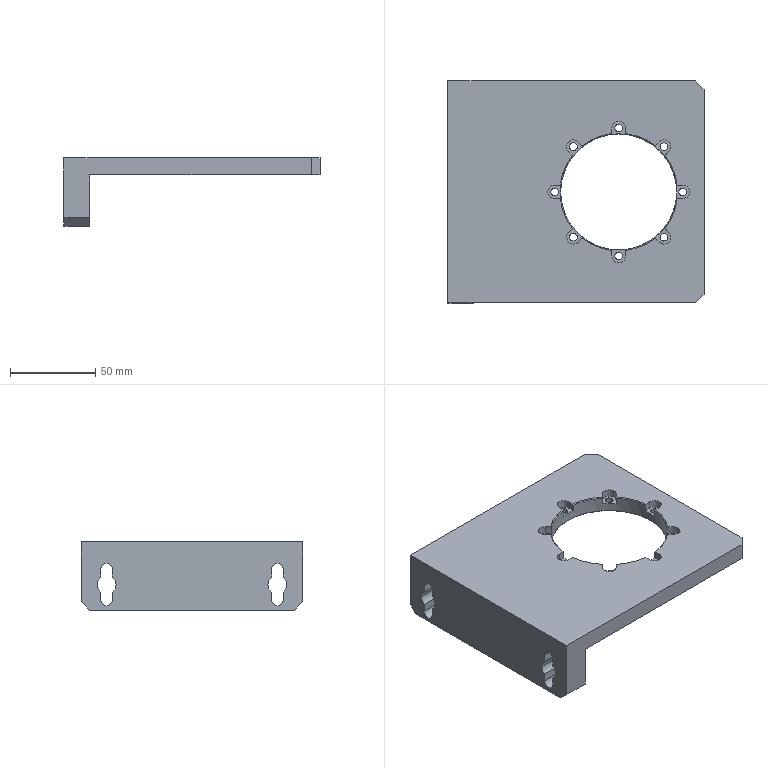NC program | NX | posted with a generic post | part box 150 x 130 x 40 mm
Lines 1321 to 2441 of 2441:
(ZLEVEL_PROFILE , TOOL : D6)
N2610 T12 M6
N2612 G54
N2614 G17 G0 G90 X55.46 Y0. B0. C0. S9500 M3
N2616 G43 Z30. H12
N2618 Z-0.46
N2620 G94 G1 X56.598 Y-0.705 F2000.
N2622 G3 X57.119 Y-1.004 R0.6
N2624 G1 X58.842 Y-1.
N2626 X62.5
N2628 G3 X63.5 Y0. R1.
N2630 X62.5 Y1. R1.
N2632 G1 X58.764 Y1.003
N2634 X57.118 Y1.004
N2636 G3 X56.598 Y0.704 R0.6
N2638 G1 X55.46 Y0.
N2640 G0 X55.455 Z-0.92
N2642 G1 X56.571 Y-0.704
N2644 G3 X57.091 Y-1.003 R0.6
N2646 G1 X58.842 Y-1.
N2648 X62.5
N2650 G3 X63.5 Y0. R1.
N2652 X62.5 Y1. R1.
N2654 G1 X58.764
N2656 X57.09 Y1.003
N2658 G3 X56.57 Y0.704 R0.6
N2660 G1 X55.455 Y0.
N2662 G0 X55.459 Z-1.38
N2664 G1 X56.543 Y-0.704
N2666 G3 X57.063 Y-1.003 R0.6
N2668 G1 X58.842 Y-1.
N2670 X62.5
N2672 G3 X63.5 Y0. R1.
N2674 X62.5 Y1. R1.
N2676 G1 X58.764
N2678 X57.062 Y1.003
N2680 G3 X56.542 Y0.704 R0.6
N2682 G1 X55.459 Y0.
N2684 G0 X55.462 Z-1.84
N2686 G1 X56.516 Y-0.703
N2688 G3 X57.036 Y-1.003 R0.6
N2690 G1 X58.842 Y-1.
N2692 X62.5
N2694 G3 X63.5 Y0. R1.
N2696 X62.5 Y1. R1.
N2698 G1 X58.764
N2700 X57.034 Y1.003
N2702 G3 X56.514 Y0.703 R0.6
N2704 G1 X55.462 Y0.
N2706 G0 X55.465 Z-2.3
N2708 G1 X56.488 Y-0.703
N2710 G3 X57.008 Y-1.002 R0.6
N2712 G1 X58.842 Y-1.
N2714 X62.5
N2716 G3 X63.5 Y0. R1.
N2718 X62.5 Y1. R1.
N2720 G1 X58.764
N2722 X57.007 Y1.002
N2724 G3 X56.487 Y0.703 R0.6
N2726 G1 X55.465 Y0.
N2728 G0 X55.467 Z-2.76
N2730 G1 X56.46 Y-0.703
N2732 G3 X56.98 Y-1.002 R0.6
N2734 G1 X58.842 Y-1.
N2736 X62.5
N2738 G3 X63.5 Y0. R1.
N2740 X62.5 Y1. R1.
N2742 G1 X58.764
N2744 X56.979 Y1.002
N2746 G3 X56.459 Y0.703 R0.6
N2748 G1 X55.467 Y0.
N2750 G0 X55.47 Z-3.22
N2752 G1 X56.433 Y-0.702
N2754 G3 X56.953 Y-1.002 R0.6
N2756 G1 X58.842 Y-1.
N2758 X62.5
N2760 G3 X63.5 Y0. R1.
N2762 X62.5 Y1. R1.
N2764 G1 X58.764
N2766 X56.951 Y1.002
N2768 G3 X56.431 Y0.702 R0.6
N2770 G1 X55.47 Y0.
N2772 G0 X55.471 Z-3.68
N2774 G1 X56.405 Y-0.702
N2776 G3 X56.925 Y-1.001 R0.6
N2778 G1 X58.842 Y-1.
N2780 X62.5
N2782 G3 X63.5 Y0. R1.
N2784 X62.5 Y1. R1.
N2786 G1 X58.764
N2788 X56.923 Y1.001
N2790 G3 X56.403 Y0.702 R0.6
N2792 G1 X55.471 Y0.
N2794 G0 X55.472 Z-4.14
N2796 G1 X56.377 Y-0.701
N2798 G3 X56.897 Y-1.001 R0.6
N2800 G1 X58.88 Y-1.
N2802 X62.5
N2804 G3 X63.5 Y0. R1.
N2806 X62.5 Y1. R1.
N2808 G1 X58.764
N2810 X56.895 Y1.001
N2812 G3 X56.375 Y0.701 R0.6
N2814 G1 X55.472 Y0.
N2816 G0 X55.471 Z-4.6
N2818 G1 X56.35 Y-0.701
N2820 G3 X56.87 Y-1.001 R0.6
N2822 G1 X58.88 Y-1.
N2824 X62.5
N2826 G3 X63.5 Y0. R1.
N2828 X62.5 Y1. R1.
N2830 G1 X58.764
N2832 X56.867 Y1.001
N2834 G3 X56.348 Y0.701 R0.6
N2836 G1 X55.471 Y0.
N2838 G0 Z30.
N2840 X46.559 Y21.559
N2842 Z-0.46
N2844 G1 X47.579 Y21.583
N2846 G3 X48.158 Y21.74 R0.6
N2848 G1 X49.644 Y23.229
N2850 X52.224 Y25.809
N2852 G3 X52.224 Y27.224 R1.
N2854 X50.809 Y27.224 R1.
N2856 G1 X48.19 Y24.604
N2858 X48.165 Y24.584
N2860 X46.741 Y23.16
N2862 G3 X46.586 Y22.58 R0.6
N2864 G1 X46.559 Y21.559
N2866 G0 X46.558 Y21.558 Z-0.92
N2868 G1 X47.579 Y21.584
N2870 G3 X48.158 Y21.74 R0.6
N2872 G1 X49.644 Y23.229
N2874 X52.224 Y25.809
N2876 G3 X52.224 Y27.224 R1.
N2878 X50.809 Y27.224 R1.
N2880 G1 X48.168 Y24.582
N2882 X46.742 Y23.159
N2884 G3 X46.586 Y22.58 R0.6
N2886 G1 X46.558 Y21.558
N2888 G0 X46.557 Y21.557 Z-1.38
N2890 G1 X47.578 Y21.584
N2892 G3 X48.158 Y21.74 R0.6
N2894 G1 X49.644 Y23.229
N2896 X52.224 Y25.809
N2898 G3 X52.224 Y27.224 R1.
N2900 X50.809 Y27.224 R1.
N2902 G1 X48.168 Y24.582
N2904 X46.742 Y23.159
N2906 G3 X46.586 Y22.58 R0.6
N2908 G1 X46.557 Y21.557
N2910 G0 X46.556 Y21.556 Z-1.84
N2912 G1 X47.578 Y21.585
N2914 G3 X48.157 Y21.74 R0.6
N2916 G1 X49.644 Y23.229
N2918 X52.224 Y25.809
N2920 G3 X52.224 Y27.224 R1.
N2922 X50.809 Y27.224 R1.
N2924 G1 X48.168 Y24.582
N2926 X46.753 Y23.169
N2928 G3 X46.597 Y22.59 R0.6
N2930 G1 X46.556 Y21.556
N2932 G0 X46.555 Y21.555 Z-2.3
N2934 G1 X47.578 Y21.585
N2936 G3 X48.157 Y21.741 R0.6
N2938 G1 X49.665 Y23.251
N2940 X52.224 Y25.809
N2942 G3 X52.224 Y27.224 R1.
N2944 X50.809 Y27.224 R1.
N2946 G1 X48.168 Y24.582
N2948 X46.753 Y23.169
N2950 G3 X46.598 Y22.589 R0.6
N2952 G1 X46.555 Y21.555
N2954 G0 X46.554 Y21.553 Z-2.76
N2956 G1 X47.577 Y21.586
N2958 G3 X48.157 Y21.741 R0.6
N2960 G1 X49.665 Y23.251
N2962 X52.224 Y25.809
N2964 G3 X52.224 Y27.224 R1.
N2966 X50.809 Y27.224 R1.
N2968 G1 X48.168 Y24.582
N2970 X46.754 Y23.168
N2972 G3 X46.598 Y22.589 R0.6
N2974 G1 X46.554 Y21.553
N2976 G0 X46.55 Y21.551 Z-3.22
N2978 G1 X47.577 Y21.586
N2980 G3 X48.156 Y21.741 R0.6
N2982 G1 X49.665 Y23.251
N2984 X52.224 Y25.809
N2986 G3 X52.224 Y27.224 R1.
N2988 X50.809 Y27.224 R1.
N2990 G1 X48.168 Y24.582
N2992 X46.754 Y23.168
N2994 G3 X46.599 Y22.588 R0.6
N2996 G1 X46.55 Y21.551
N2998 G0 X46.549 Y21.55 Z-3.68
N3000 G1 X47.576 Y21.586
N3002 G3 X48.156 Y21.742 R0.6
N3004 G1 X49.665 Y23.251
N3006 X52.224 Y25.809
N3008 G3 X52.224 Y27.224 R1.
N3010 X50.809 Y27.224 R1.
N3012 G1 X48.168 Y24.582
N3014 X46.754 Y23.168
N3016 G3 X46.599 Y22.588 R0.6
N3018 G1 X46.549 Y21.55
N3020 G0 X46.55 Z-4.14
N3022 G1 X47.576 Y21.587
N3024 G3 X48.156 Y21.742 R0.6
N3026 G1 X49.665 Y23.251
N3028 X52.224 Y25.809
N3030 G3 X52.224 Y27.224 R1.
N3032 X50.809 Y27.224 R1.
N3034 G1 X48.168 Y24.582
N3036 X46.755 Y23.167
N3038 G3 X46.6 Y22.588 R0.6
N3040 G1 X46.55 Y21.55
N3042 G0 X46.548 Y21.548 Z-4.6
N3044 G1 X47.586 Y21.598
N3046 G3 X48.166 Y21.753 R0.6
N3048 G1 X49.665 Y23.251
N3050 X52.224 Y25.809
N3052 G3 X52.224 Y27.224 R1.
N3054 X50.809 Y27.224 R1.
N3056 G1 X48.168 Y24.582
N3058 X46.755 Y23.167
N3060 G3 X46.6 Y22.587 R0.6
N3062 G1 X46.548 Y21.548
N3064 G0 Z30.
N3066 X25. Y30.46
N3068 Z-0.46
N3070 G1 X25.705 Y31.598
N3072 G3 X26.004 Y32.118 R0.6
N3074 G1 X26. Y33.991
N3076 Y37.5
N3078 G3 X25. Y38.5 R1.
N3080 X24. Y37.5 R1.
N3082 G1 Y33.991
N3084 X23.996 Y32.118
N3086 G3 X24.295 Y31.598 R0.6
N3088 G1 X25. Y30.46
N3090 G0 Y30.454 Z-0.92
N3092 G1 X25.704 Y31.57
N3094 G3 X26.003 Y32.09 R0.6
N3096 G1 X26. Y33.991
N3098 Y37.5
N3100 G3 X25. Y38.5 R1.
N3102 X24. Y37.5 R1.
N3104 G1 Y33.991
N3106 X23.997 Y32.09
N3108 G3 X24.296 Y31.57 R0.6
N3110 G1 X25. Y30.454
N3112 G0 Y30.459 Z-1.38
N3114 G1 X25.704 Y31.542
N3116 G3 X26.003 Y32.062 R0.6
N3118 G1 X26. Y33.991
N3120 Y37.5
N3122 G3 X25. Y38.5 R1.
N3124 X24. Y37.5 R1.
N3126 G1 Y33.991
N3128 X23.997 Y32.062
N3130 G3 X24.296 Y31.542 R0.6
N3132 G1 X25. Y30.459
N3134 G0 Y30.462 Z-1.84
N3136 G1 X25.703 Y31.514
N3138 G3 X26.003 Y32.034 R0.6
N3140 G1 X26. Y33.991
N3142 Y37.5
N3144 G3 X25. Y38.5 R1.
N3146 X24. Y37.5 R1.
N3148 G1 Y33.991
N3150 X23.997 Y32.034
N3152 G3 X24.297 Y31.514 R0.6
N3154 G1 X25. Y30.462
N3156 G0 Y30.466 Z-2.3
N3158 G1 X25.703 Y31.487
N3160 G3 X26.002 Y32.007 R0.6
N3162 G1 X26. Y33.991
N3164 Y37.5
N3166 G3 X25. Y38.5 R1.
N3168 X24. Y37.5 R1.
N3170 G1 Y33.991
N3172 X23.998 Y32.007
N3174 G3 X24.297 Y31.487 R0.6
N3176 G1 X25. Y30.466
N3178 G0 Y30.467 Z-2.76
N3180 G1 X25.702 Y31.459
N3182 G3 X26.002 Y31.979 R0.6
N3184 G1 X26. Y33.991
N3186 Y37.5
N3188 G3 X25. Y38.5 R1.
N3190 X24. Y37.5 R1.
N3192 G1 Y33.991
N3194 X23.998 Y31.979
N3196 G3 X24.298 Y31.459 R0.6
N3198 G1 X25. Y30.467
N3200 G0 Y30.47 Z-3.22
N3202 G1 X25.702 Y31.431
N3204 G3 X26.002 Y31.951 R0.6
N3206 G1 X26. Y33.991
N3208 Y37.5
N3210 G3 X25. Y38.5 R1.
N3212 X24. Y37.5 R1.
N3214 G1 Y33.991
N3216 X23.998 Y31.951
N3218 G3 X24.298 Y31.431 R0.6
N3220 G1 X25. Y30.47
N3222 G0 Y30.471 Z-3.68
N3224 G1 X25.702 Y31.403
N3226 G3 X26.001 Y31.923 R0.6
N3228 G1 X26. Y33.991
N3230 Y37.5
N3232 G3 X25. Y38.5 R1.
N3234 X24. Y37.5 R1.
N3236 G1 Y33.991
N3238 X23.999 Y31.923
N3240 G3 X24.298 Y31.403 R0.6
N3242 G1 X25. Y30.471
N3244 G0 Y30.472 Z-4.14
N3246 G1 X25.701 Y31.375
N3248 G3 X26.001 Y31.895 R0.6
N3250 G1 X26. Y33.991
N3252 Y37.5
N3254 G3 X25. Y38.5 R1.
N3256 X24. Y37.5 R1.
N3258 G1 Y33.991
N3260 X23.999 Y31.895
N3262 G3 X24.299 Y31.375 R0.6
N3264 G1 X25. Y30.472
N3266 G0 Y30.471 Z-4.6
N3268 G1 X25.701 Y31.348
N3270 G3 X26.001 Y31.867 R0.6
N3272 G1 X26. Y33.991
N3274 Y37.5
N3276 G3 X25. Y38.5 R1.
N3278 X24. Y37.5 R1.
N3280 G1 Y33.991
N3282 X23.999 Y31.867
N3284 G3 X24.299 Y31.348 R0.6
N3286 G1 X25. Y30.471
N3288 G0 Z30.
N3290 X3.439 Y21.56
N3292 Z-0.46
N3294 G1 X3.416 Y22.579
N3296 G3 X3.26 Y23.159 R0.6
N3298 G1 X1.939 Y24.48
N3300 X1.821 Y24.593
N3302 X-0.809 Y27.224
N3304 G3 X-2.224 Y27.224 R1.
N3306 X-2.224 Y25.809 R1.
N3308 G1 X0.396 Y23.19
N3310 X0.416 Y23.165
N3312 X1.84 Y21.74
N3314 G3 X2.42 Y21.584 R0.6
N3316 G1 X3.439 Y21.56
N3318 G0 X3.44 Y21.559 Z-0.92
N3320 G1 X3.415 Y22.579
N3322 G3 X3.26 Y23.158 R0.6
N3324 G1 X1.96 Y24.458
N3326 X1.832 Y24.582
N3328 X-0.809 Y27.224
N3330 G3 X-2.224 Y27.224 R1.
N3332 X-2.224 Y25.809 R1.
N3334 G1 X0.418 Y23.168
N3336 X1.84 Y21.74
N3338 G3 X2.42 Y21.584 R0.6
N3340 G1 X3.44 Y21.559
N3342 G0 X3.442 Y21.558 Z-1.38
N3344 G1 X3.415 Y22.579
N3346 G3 X3.26 Y23.158 R0.6
N3348 G1 X1.959 Y24.458
N3350 X1.832 Y24.582
N3352 X-0.809 Y27.224
N3354 G3 X-2.224 Y27.224 R1.
N3356 X-2.224 Y25.809 R1.
N3358 G1 X0.418 Y23.168
N3360 X1.841 Y21.741
N3362 G3 X2.42 Y21.584 R0.6
N3364 G1 X3.442 Y21.558
N3366 G0 X3.443 Y21.557 Z-1.84
N3368 G1 X3.415 Y22.578
N3370 G3 X3.259 Y23.158 R0.6
N3372 G1 X1.832 Y24.582
N3374 X-0.809 Y27.224
N3376 G3 X-2.224 Y27.224 R1.
N3378 X-2.224 Y25.809 R1.
N3380 G1 X0.418 Y23.168
N3382 X1.841 Y21.741
N3384 G3 X2.42 Y21.585 R0.6
N3386 G1 X3.443 Y21.557
N3388 G0 X3.444 Y21.556 Z-2.3
N3390 G1 X3.415 Y22.578
N3392 G3 X3.259 Y23.157 R0.6
N3394 G1 X1.832 Y24.582
N3396 X-0.809 Y27.224
N3398 G3 X-2.224 Y27.224 R1.
N3400 X-2.224 Y25.809 R1.
N3402 G1 X0.418 Y23.168
N3404 X1.841 Y21.741
N3406 G3 X2.421 Y21.585 R0.6
N3408 G1 X3.444 Y21.556
N3410 G0 X3.445 Y21.555 Z-2.76
N3412 G1 X3.414 Y22.578
N3414 G3 X3.259 Y23.157 R0.6
N3416 G1 X1.832 Y24.582
N3418 X-0.809 Y27.224
N3420 G3 X-2.224 Y27.224 R1.
N3422 X-2.224 Y25.809 R1.
N3424 G1 X0.418 Y23.168
N3426 X1.842 Y21.741
N3428 G3 X2.421 Y21.586 R0.6
N3430 G1 X3.445 Y21.555
N3432 G0 X3.447 Y21.551 Z-3.22
N3434 G1 X3.414 Y22.577
N3436 G3 X3.259 Y23.157 R0.6
N3438 G1 X1.832 Y24.582
N3440 X-0.809 Y27.224
N3442 G3 X-2.224 Y27.224 R1.
N3444 X-2.224 Y25.809 R1.
N3446 G1 X0.418 Y23.168
N3448 X1.842 Y21.742
N3450 G3 X2.422 Y21.586 R0.6
N3452 G1 X3.447 Y21.551
N3454 G0 X3.448 Y21.55 Z-3.68
N3456 G1 X3.403 Y22.587
N3458 G3 X3.247 Y23.167 R0.6
N3460 G1 X1.832 Y24.582
N3462 X-0.809 Y27.224
N3464 G3 X-2.224 Y27.224 R1.
N3466 X-2.224 Y25.809 R1.
N3468 G1 X0.418 Y23.168
N3470 X1.843 Y21.742
N3472 G3 X2.422 Y21.587 R0.6
N3474 G1 X3.448 Y21.55
N3476 G0 X3.449 Y21.551 Z-4.14
N3478 G1 X3.402 Y22.587
N3480 G3 X3.247 Y23.167 R0.6
N3482 G1 X1.832 Y24.582
N3484 X-0.809 Y27.224
N3486 G3 X-2.224 Y27.224 R1.
N3488 X-2.224 Y25.809 R1.
N3490 G1 X0.418 Y23.168
N3492 X1.832 Y21.753
N3494 G3 X2.412 Y21.598 R0.6
N3496 G1 X3.449 Y21.551
N3498 G0 X3.45 Y21.55 Z-4.6
N3500 G1 X3.402 Y22.587
N3502 G3 X3.247 Y23.166 R0.6
N3504 G1 X1.832 Y24.582
N3506 X-0.809 Y27.224
N3508 G3 X-2.224 Y27.224 R1.
N3510 X-2.224 Y25.809 R1.
N3512 G1 X0.418 Y23.168
N3514 X1.833 Y21.753
N3516 G3 X2.412 Y21.598 R0.6
N3518 G1 X3.45 Y21.55
N3520 G0 Z30.
N3522 X-5.46 Y0.
N3524 Z-0.46
N3526 G1 X-6.599 Y0.705
N3528 G3 X-7.119 Y1.004 R0.6
N3530 G1 X-8.742 Y1.
N3532 X-12.5
N3534 G3 X-13.5 Y0. R1.
N3536 X-12.5 Y-1. R1.
N3538 G1 X-8.764 Y-1.003
N3540 X-7.118 Y-1.004
N3542 G3 X-6.598 Y-0.704 R0.6
N3544 G1 X-5.46 Y0.
N3546 G0 X-5.462 Y0.002 Z-0.92
N3548 G1 X-6.571 Y0.704
N3550 G3 X-7.091 Y1.003 R0.6
N3552 G1 X-8.718 Y1.
N3554 X-12.5
N3556 G3 X-13.5 Y0. R1.
N3558 X-12.5 Y-1. R1.
N3560 G1 X-8.764
N3562 X-8.182 Y-1.057
N3564 X-8.134 Y-1.002
N3566 X-7.09 Y-1.003
N3568 G3 X-6.57 Y-0.704 R0.6
N3570 G1 X-5.462 Y0.002
N3572 G0 X-5.465 Y0.001 Z-1.38
N3574 G1 X-6.543 Y0.704
N3576 G3 X-7.063 Y1.003 R0.6
N3578 G1 X-8.718 Y1.
N3580 X-12.5
N3582 G3 X-13.5 Y0. R1.
N3584 X-12.5 Y-1. R1.
N3586 G1 X-8.764
N3588 X-8.182 Y-1.057
N3590 X-8.134 Y-1.002
N3592 X-7.062 Y-1.003
N3594 G3 X-6.543 Y-0.703 R0.6
N3596 G1 X-5.465 Y0.001
N3598 G0 X-5.468 Z-1.84
N3600 G1 X-6.516 Y0.703
N3602 G3 X-7.036 Y1.003 R0.6
N3604 G1 X-8.718 Y1.
N3606 X-12.5
N3608 G3 X-13.5 Y0. R1.
N3610 X-12.5 Y-1. R1.
N3612 G1 X-8.764
N3614 X-8.182 Y-1.057
N3616 X-8.134 Y-1.002
N3618 X-7.035 Y-1.003
N3620 G3 X-6.515 Y-0.703 R0.6
N3622 G1 X-5.468 Y0.001
N3624 G0 X-5.469 Z-2.3
N3626 G1 X-6.488 Y0.703
N3628 G3 X-7.008 Y1.002 R0.6
N3630 G1 X-8.718 Y1.
N3632 X-12.5
N3634 G3 X-13.5 Y0. R1.
N3636 X-12.5 Y-1. R1.
N3638 G1 X-8.764
N3640 X-8.182 Y-1.057
N3642 X-8.134 Y-1.001
N3644 X-7.007 Y-1.002
N3646 G3 X-6.487 Y-0.703 R0.6
N3648 G1 X-5.469 Y0.001
N3650 G0 X-5.471 Y0. Z-2.76
N3652 G1 X-6.46 Y0.703
N3654 G3 X-6.98 Y1.002 R0.6
N3656 G1 X-8.718 Y1.
N3658 X-12.5
N3660 G3 X-13.5 Y0. R1.
N3662 X-12.5 Y-1. R1.
N3664 G1 X-8.764
N3666 X-8.182 Y-1.057
N3668 X-8.134 Y-1.001
N3670 X-6.979 Y-1.002
N3672 G3 X-6.459 Y-0.703 R0.6
N3674 G1 X-5.471 Y0.
N3676 G0 X-5.473 Z-3.22
N3678 G1 X-6.433 Y0.702
N3680 G3 X-6.953 Y1.002 R0.6
N3682 G1 X-8.718 Y1.
N3684 X-12.5
N3686 G3 X-13.5 Y0. R1.
N3688 X-12.5 Y-1. R1.
N3690 G1 X-8.764
N3692 X-8.182 Y-1.057
N3694 X-8.134 Y-1.
N3696 X-6.951 Y-1.002
N3698 G3 X-6.431 Y-0.702 R0.6
N3700 G1 X-5.473 Y0.
N3702 G0 X-5.476 Y-0.001 Z-3.68
N3704 G1 X-6.405 Y0.702
N3706 G3 X-6.925 Y1.001 R0.6
N3708 G1 X-8.718 Y1.
N3710 X-12.5
N3712 G3 X-13.5 Y0. R1.
N3714 X-12.5 Y-1. R1.
N3716 G1 X-8.764
N3718 X-8.182 Y-1.057
N3720 X-8.134 Y-1.
N3722 X-6.923 Y-1.001
N3724 G3 X-6.403 Y-0.702 R0.6
N3726 G1 X-5.476 Y-0.001
N3728 G0 X-5.475 Z-4.14
N3730 G1 X-6.378 Y0.701
N3732 G3 X-6.897 Y1.001 R0.6
N3734 G1 X-8.821 Y1.
N3736 X-12.5
N3738 G3 X-13.5 Y0. R1.
N3740 X-12.5 Y-1. R1.
N3742 G1 X-8.764
N3744 X-8.182 Y-1.057
N3746 X-8.134 Y-1.
N3748 X-6.895 Y-1.001
N3750 G3 X-6.375 Y-0.702 R0.6
N3752 G1 X-5.475 Y-0.001
N3754 G0 X-5.457 Y-0.005 Z-4.6
N3756 G1 X-6.35 Y0.701
N3758 G3 X-6.87 Y1.001 R0.6
N3760 G1 X-8.821 Y1.
N3762 X-12.5
N3764 G3 X-13.5 Y0. R1.
N3766 X-12.5 Y-1. R1.
N3768 G1 X-8.764 Y-0.999
N3770 X-8.182 Y-1.057
N3772 X-8.134 Y-0.999
N3774 X-6.868 Y-1.001
N3776 G3 X-6.348 Y-0.701 R0.6
N3778 G1 X-5.457 Y-0.005
N3780 G0 Z30.
N3782 X3.441 Y-21.559
N3784 Z-0.46
N3786 G1 X2.42 Y-21.586
N3788 G3 X1.84 Y-21.741 R0.6
N3790 G1 X0.416 Y-23.165
N3792 X0.396 Y-23.19
N3794 X-2.224 Y-25.809
N3796 G3 X-2.224 Y-27.224 R1.
N3798 X-0.809 Y-27.224 R1.
N3800 G1 X1.81 Y-24.604
N3802 X1.835 Y-24.584
N3804 X3.234 Y-23.184
N3806 G3 X3.389 Y-22.605 R0.6
N3808 G1 X3.441 Y-21.559
N3810 G0 X3.442 Y-21.558 Z-0.92
N3812 G1 X2.42 Y-21.586
N3814 G3 X1.841 Y-21.742 R0.6
N3816 G1 X0.452 Y-23.134
N3818 X-2.224 Y-25.809
N3820 G3 X-2.224 Y-27.224 R1.
N3822 X-0.809 Y-27.224 R1.
N3824 G1 X1.832 Y-24.582
N3826 X2.278 Y-24.215
N3828 X2.27 Y-24.146
N3830 X3.234 Y-23.184
N3832 G3 X3.389 Y-22.605 R0.6
N3834 G1 X3.442 Y-21.558
N3836 G0 X3.443 Y-21.557 Z-1.38
N3838 G1 X2.42 Y-21.586
N3840 G3 X1.841 Y-21.742 R0.6
N3842 G1 X0.452 Y-23.134
N3844 X-2.224 Y-25.809
N3846 G3 X-2.224 Y-27.224 R1.
N3848 X-0.809 Y-27.224 R1.
N3850 G1 X1.832 Y-24.582
N3852 X2.278 Y-24.215
N3854 X2.27 Y-24.146
N3856 X3.234 Y-23.184
N3858 G3 X3.389 Y-22.604 R0.6
N3860 G1 X3.443 Y-21.557
N3862 G0 X3.444 Y-21.556 Z-1.84
N3864 G1 X2.421 Y-21.587
N3866 G3 X1.841 Y-21.742 R0.6
N3868 G1 X0.452 Y-23.134
N3870 X-2.224 Y-25.809
N3872 G3 X-2.224 Y-27.224 R1.
N3874 X-0.809 Y-27.224 R1.
N3876 G1 X1.832 Y-24.582
N3878 X2.278 Y-24.215
N3880 X2.27 Y-24.145
N3882 X3.234 Y-23.183
N3884 G3 X3.389 Y-22.604 R0.6
N3886 G1 X3.444 Y-21.556
N3888 G0 X3.448 Y-21.553 Z-2.3
N3890 G1 X2.421 Y-21.587
N3892 G3 X1.842 Y-21.743 R0.6
N3894 G1 X0.452 Y-23.134
N3896 X-2.224 Y-25.809
N3898 G3 X-2.224 Y-27.224 R1.
N3900 X-0.809 Y-27.224 R1.
N3902 G1 X1.832 Y-24.582
N3904 X2.278 Y-24.215
N3906 X2.269 Y-24.145
N3908 X3.234 Y-23.183
N3910 G3 X3.389 Y-22.603 R0.6
N3912 G1 X3.448 Y-21.553
N3914 G0 X3.446 Y-21.554 Z-2.76
N3916 G1 X2.422 Y-21.587
N3918 G3 X1.842 Y-21.743 R0.6
N3920 G1 X0.452 Y-23.134
N3922 X-2.224 Y-25.809
N3924 G3 X-2.224 Y-27.224 R1.
N3926 X-0.809 Y-27.224 R1.
N3928 G1 X1.832 Y-24.582
N3930 X2.278 Y-24.215
N3932 X2.269 Y-24.145
N3934 X3.234 Y-23.182
N3936 G3 X3.389 Y-22.603 R0.6
N3938 G1 X3.446 Y-21.554
N3940 G0 X3.45 Y-21.551 Z-3.22
N3942 G1 X2.422 Y-21.588
N3944 G3 X1.842 Y-21.743 R0.6
N3946 G1 X0.452 Y-23.134
N3948 X-2.224 Y-25.809
N3950 G3 X-2.224 Y-27.224 R1.
N3952 X-0.809 Y-27.224 R1.
N3954 G1 X1.832 Y-24.582
N3956 X2.278 Y-24.215
N3958 X2.269 Y-24.145
N3960 X3.234 Y-23.182
N3962 G3 X3.389 Y-22.602 R0.6
N3964 G1 X3.45 Y-21.551
N3966 G0 X3.451 Z-3.68
N3968 G1 X2.412 Y-21.599
N3970 G3 X1.832 Y-21.754 R0.6
N3972 G1 X0.452 Y-23.134
N3974 X-2.224 Y-25.809
N3976 G3 X-2.224 Y-27.224 R1.
N3978 X-0.809 Y-27.224 R1.
N3980 G1 X1.832 Y-24.582
N3982 X2.278 Y-24.215
N3984 X2.269 Y-24.144
N3986 X3.234 Y-23.181
N3988 G3 X3.389 Y-22.602 R0.6
N3990 G1 X3.451 Y-21.551
N3992 G0 X3.452 Y-21.549 Z-4.14
N3994 G1 X2.412 Y-21.6
N3996 G3 X1.833 Y-21.755 R0.6
N3998 G1 X0.452 Y-23.134
N4000 X-2.224 Y-25.809
N4002 G3 X-2.224 Y-27.224 R1.
N4004 X-0.809 Y-27.224 R1.
N4006 G1 X1.832 Y-24.582
N4008 X2.278 Y-24.215
N4010 X2.268 Y-24.144
N4012 X3.234 Y-23.181
N4014 G3 X3.39 Y-22.601 R0.6
N4016 G1 X3.452 Y-21.549
N4018 G0 X3.453 Y-21.548 Z-4.6
N4020 G1 X2.413 Y-21.6
N4022 G3 X1.833 Y-21.755 R0.6
N4024 G1 X0.396 Y-23.19
N4026 X-2.224 Y-25.809
N4028 G3 X-2.224 Y-27.224 R1.
N4030 X-0.809 Y-27.224 R1.
N4032 G1 X1.832 Y-24.582
N4034 X2.278 Y-24.215
N4036 X2.268 Y-24.144
N4038 X3.234 Y-23.18
N4040 G3 X3.39 Y-22.601 R0.6
N4042 G1 X3.453 Y-21.548
N4044 G0 Z30.
N4046 X25. Y-30.46
N4048 Z-0.46
N4050 G1 X24.295 Y-31.598
N4052 G3 X23.996 Y-32.118 R0.6
N4054 G1 X24. Y-33.742
N4056 Y-37.5
N4058 G3 X25. Y-38.5 R1.
N4060 X26. Y-37.5 R1.
N4062 G1 X26.003 Y-33.764
N4064 X26.004 Y-32.118
N4066 G3 X25.704 Y-31.598 R0.6
N4068 G1 X25. Y-30.46
N4070 G0 X24.998 Y-30.462 Z-0.92
N4072 G1 X24.296 Y-31.57
N4074 G3 X23.997 Y-32.09 R0.6
N4076 G1 X24. Y-33.718
N4078 Y-37.5
N4080 G3 X25. Y-38.5 R1.
N4082 X26. Y-37.5 R1.
N4084 G1 Y-33.764
N4086 X26.057 Y-33.182
N4088 X26.002 Y-33.134
N4090 X26.003 Y-32.09
N4092 G3 X25.704 Y-31.57 R0.6
N4094 G1 X24.998 Y-30.462
N4096 G0 X24.999 Y-30.465 Z-1.38
N4098 G1 X24.296 Y-31.542
N4100 G3 X23.997 Y-32.062 R0.6
N4102 G1 X24. Y-33.718
N4104 Y-37.5
N4106 G3 X25. Y-38.5 R1.
N4108 X26. Y-37.5 R1.
N4110 G1 Y-33.764
N4112 X26.057 Y-33.182
N4114 X26.002 Y-33.134
N4116 X26.003 Y-32.062
N4118 G3 X25.703 Y-31.543 R0.6
N4120 G1 X24.999 Y-30.465
N4122 G0 Y-30.468 Z-1.84
N4124 G1 X24.297 Y-31.515
N4126 G3 X23.997 Y-32.035 R0.6
N4128 G1 X24. Y-33.718
N4130 Y-37.5
N4132 G3 X25. Y-38.5 R1.
N4134 X26. Y-37.5 R1.
N4136 G1 Y-33.764
N4138 X26.057 Y-33.182
N4140 X26.002 Y-33.134
N4142 X26.003 Y-32.035
N4144 G3 X25.703 Y-31.515 R0.6
N4146 G1 X24.999 Y-30.468
N4148 G0 Y-30.469 Z-2.3
N4150 G1 X24.297 Y-31.487
N4152 G3 X23.998 Y-32.007 R0.6
N4154 G1 X24. Y-33.718
N4156 Y-37.5
N4158 G3 X25. Y-38.5 R1.
N4160 X26. Y-37.5 R1.
N4162 G1 Y-33.764
N4164 X26.057 Y-33.182
N4166 X26.001 Y-33.134
N4168 X26.002 Y-32.007
N4170 G3 X25.703 Y-31.487 R0.6
N4172 G1 X24.999 Y-30.469
N4174 G0 X25. Y-30.471 Z-2.76
N4176 G1 X24.297 Y-31.459
N4178 G3 X23.998 Y-31.979 R0.6
N4180 G1 X24. Y-33.718
N4182 Y-37.5
N4184 G3 X25. Y-38.5 R1.
N4186 X26. Y-37.5 R1.
N4188 G1 Y-33.764
N4190 X26.057 Y-33.182
N4192 X26.001 Y-33.134
N4194 X26.002 Y-31.979
N4196 G3 X25.703 Y-31.459 R0.6
N4198 G1 X25. Y-30.471
N4200 G0 Y-30.473 Z-3.22
N4202 G1 X24.298 Y-31.431
N4204 G3 X23.998 Y-31.951 R0.6
N4206 G1 X24. Y-33.718
N4208 Y-37.5
N4210 G3 X25. Y-38.5 R1.
N4212 X26. Y-37.5 R1.
N4214 G1 Y-33.764
N4216 X26.057 Y-33.182
N4218 X26. Y-33.134
N4220 X26.002 Y-31.951
N4222 G3 X25.702 Y-31.431 R0.6
N4224 G1 X25. Y-30.473
N4226 G0 X25.001 Y-30.476 Z-3.68
N4228 G1 X24.298 Y-31.403
N4230 G3 X23.999 Y-31.923 R0.6
N4232 G1 X24. Y-33.718
N4234 Y-37.5
N4236 G3 X25. Y-38.5 R1.
N4238 X26. Y-37.5 R1.
N4240 G1 Y-33.764
N4242 X26.057 Y-33.182
N4244 X26. Y-33.134
N4246 X26.001 Y-31.923
N4248 G3 X25.702 Y-31.403 R0.6
N4250 G1 X25.001 Y-30.476
N4252 G0 Y-30.475 Z-4.14
N4254 G1 X24.299 Y-31.375
N4256 G3 X23.999 Y-31.895 R0.6
N4258 G1 X24. Y-33.821
N4260 Y-37.5
N4262 G3 X25. Y-38.5 R1.
N4264 X26. Y-37.5 R1.
N4266 G1 Y-33.764
N4268 X26.057 Y-33.182
N4270 X26. Y-33.134
N4272 X26.001 Y-31.895
N4274 G3 X25.702 Y-31.375 R0.6
N4276 G1 X25.001 Y-30.475
N4278 G0 X25.005 Y-30.457 Z-4.6
N4280 G1 X24.299 Y-31.348
N4282 G3 X23.999 Y-31.868 R0.6
N4284 G1 X24. Y-33.821
N4286 Y-37.5
N4288 G3 X25. Y-38.5 R1.
N4290 X26. Y-37.5 R1.
N4292 G1 X25.999 Y-33.764
N4294 X26.057 Y-33.182
N4296 X25.999 Y-33.134
N4298 X26.001 Y-31.868
N4300 G3 X25.701 Y-31.348 R0.6
N4302 G1 X25.005 Y-30.457
N4304 G0 Z30.
N4306 X46.56 Y-21.56
N4308 Z-0.46
N4310 G1 X46.586 Y-22.58
N4312 G3 X46.741 Y-23.16 R0.6
N4314 G1 X48.165 Y-24.584
N4316 X48.19 Y-24.604
N4318 X50.809 Y-27.224
N4320 G3 X52.224 Y-27.224 R1.
N4322 X52.224 Y-25.809 R1.
N4324 G1 X49.604 Y-23.19
N4326 X49.584 Y-23.165
N4328 X48.159 Y-21.74
N4330 G3 X47.58 Y-21.584 R0.6
N4332 G1 X46.56 Y-21.56
N4334 G0 X46.559 Y-21.559 Z-0.92
N4336 G1 X46.586 Y-22.58
N4338 G3 X46.742 Y-23.16 R0.6
N4340 G1 X48.134 Y-24.548
N4342 X50.809 Y-27.224
N4344 G3 X52.224 Y-27.224 R1.
N4346 X52.224 Y-25.809 R1.
N4348 G1 X49.582 Y-23.168
N4350 X49.215 Y-22.722
N4352 X49.146 Y-22.73
N4354 X48.159 Y-21.74
N4356 G3 X47.579 Y-21.584 R0.6
N4358 G1 X46.559 Y-21.559
N4360 G0 X46.558 Y-21.557 Z-1.38
N4362 G1 X46.586 Y-22.58
N4364 G3 X46.742 Y-23.159 R0.6
N4366 G1 X48.134 Y-24.548
N4368 X50.809 Y-27.224
N4370 G3 X52.224 Y-27.224 R1.
N4372 X52.224 Y-25.809 R1.
N4374 G1 X49.582 Y-23.168
N4376 X49.215 Y-22.722
N4378 X49.146 Y-22.73
N4380 X48.158 Y-21.74
N4382 G3 X47.579 Y-21.584 R0.6
N4384 G1 X46.558 Y-21.557
N4386 G0 X46.557 Y-21.556 Z-1.84
N4388 G1 X46.587 Y-22.58
N4390 G3 X46.742 Y-23.159 R0.6
N4392 G1 X48.134 Y-24.548
N4394 X50.809 Y-27.224
N4396 G3 X52.224 Y-27.224 R1.
N4398 X52.224 Y-25.809 R1.
N4400 G1 X49.582 Y-23.168
N4402 X49.215 Y-22.722
N4404 X49.205 Y-22.76
N4406 X49.166 Y-22.764
N4408 X49.147 Y-22.731
N4410 X48.158 Y-21.741
N4412 G3 X47.579 Y-21.585 R0.6
N4414 G1 X46.557 Y-21.556
N4416 G0 X46.556 Y-21.555 Z-2.3
N4418 G1 X46.587 Y-22.579
N4420 G3 X46.743 Y-23.159 R0.6
N4422 G1 X48.134 Y-24.548
N4424 X50.809 Y-27.224
N4426 G3 X52.224 Y-27.224 R1.
N4428 X52.224 Y-25.809 R1.
N4430 G1 X49.582 Y-23.168
N4432 X49.215 Y-22.722
N4434 X49.205 Y-22.76
N4436 X49.166 Y-22.765
N4438 X49.147 Y-22.731
N4440 X48.158 Y-21.741
N4442 G3 X47.578 Y-21.585 R0.6
N4444 G1 X46.556 Y-21.555
N4446 G0 X46.554 Y-21.554 Z-2.76
N4448 G1 X46.587 Y-22.579
N4450 G3 X46.743 Y-23.158 R0.6
N4452 G1 X48.134 Y-24.548
N4454 X50.809 Y-27.224
N4456 G3 X52.224 Y-27.224 R1.
N4458 X52.224 Y-25.809 R1.
N4460 G1 X49.582 Y-23.168
N4462 X49.215 Y-22.722
N4464 X49.205 Y-22.76
N4466 X49.166 Y-22.765
N4468 X49.147 Y-22.731
N4470 X48.157 Y-21.741
N4472 G3 X47.578 Y-21.586 R0.6
N4474 G1 X46.554 Y-21.554
N4476 G0 X46.552 Y-21.55 Z-3.22
N4478 G1 X46.588 Y-22.578
N4480 G3 X46.743 Y-23.158 R0.6
N4482 G1 X48.134 Y-24.548
N4484 X50.809 Y-27.224
N4486 G3 X52.224 Y-27.224 R1.
N4488 X52.224 Y-25.809 R1.
N4490 G1 X49.582 Y-23.168
N4492 X49.215 Y-22.722
N4494 X49.205 Y-22.76
N4496 X49.166 Y-22.765
N4498 X49.147 Y-22.732
N4500 X48.157 Y-21.742
N4502 G3 X47.578 Y-21.586 R0.6
N4504 G1 X46.552 Y-21.55
N4506 G0 X46.551 Y-21.549 Z-3.68
N4508 G1 X46.588 Y-22.578
N4510 G3 X46.744 Y-23.158 R0.6
N4512 G1 X48.134 Y-24.548
N4514 X50.809 Y-27.224
N4516 G3 X52.224 Y-27.224 R1.
N4518 X52.224 Y-25.809 R1.
N4520 G1 X49.582 Y-23.168
N4522 X49.215 Y-22.722
N4524 X49.205 Y-22.76
N4526 X49.166 Y-22.765
N4528 X49.147 Y-22.732
N4530 X48.157 Y-21.742
N4532 G3 X47.577 Y-21.587 R0.6
N4534 G1 X46.551 Y-21.549
N4536 G0 Y-21.55 Z-4.14
N4538 G1 X46.589 Y-22.578
N4540 G3 X46.744 Y-23.157 R0.6
N4542 G1 X48.134 Y-24.548
N4544 X50.809 Y-27.224
N4546 G3 X52.224 Y-27.224 R1.
N4548 X52.224 Y-25.809 R1.
N4550 G1 X49.582 Y-23.168
N4552 X49.215 Y-22.722
N4554 X49.206 Y-22.76
N4556 X49.167 Y-22.766
N4558 X49.147 Y-22.732
N4560 X48.156 Y-21.742
N4562 G3 X47.577 Y-21.587 R0.6
N4564 G1 X46.551 Y-21.55
N4566 G0 X46.549 Y-21.549 Z-4.6
N4568 G1 X46.589 Y-22.577
N4570 G3 X46.744 Y-23.157 R0.6
N4572 G1 X48.19 Y-24.604
N4574 X50.809 Y-27.224
N4576 G3 X52.224 Y-27.224 R1.
N4578 X52.224 Y-25.809 R1.
N4580 G1 X49.582 Y-23.168
N4582 X49.215 Y-22.722
N4584 X49.206 Y-22.76
N4586 X49.167 Y-22.766
N4588 X49.147 Y-22.733
N4590 X48.167 Y-21.753
N4592 G3 X47.587 Y-21.598 R0.6
N4594 G1 X46.549 Y-21.549
N4596 G0 Z30.
N4598 M5
(PLANAR_MILL_COPY_COPY_COPY_COPY_COPY_COPY_1 , TOOL : D6A45)
N4600 T01 M6
N4602 G54
N4604 G17 G0 G90 X-3.741 Y67.1 B0. C0. S9500 M3
N4606 G43 Z30. H1
N4608 Z0.5
N4610 G94 G1 Z-1. F1250.
N4612 X-3.337 Y66.4
N4614 G3 X-2.471 Y65.9 R1.
N4616 G1 X69.959
N4618 G2 X70.666 Y65.607 R1.
N4620 G1 X75.607 Y60.666
N4622 G2 X75.9 Y59.959 R1.
N4624 G1 Y-59.959
N4626 G2 X75.607 Y-60.666 R1.
N4628 G1 X70.666 Y-65.607
N4630 G2 X69.959 Y-65.9 R1.
N4632 G1 X-74.9
N4634 G2 X-75.9 Y-64.9 R1.
N4636 G1 Y64.9
N4638 G2 X-74.9 Y65.9 R1.
N4640 G1 X-2.471
N4642 G3 X-1.605 Y66.4 R1.
N4644 G1 X-1.201 Y67.1
N4646 Z0.5
N4648 G0 Z30.
N4650 X26.9 Y34.406
N4652 Z0.5
N4654 G1 Z-1.
N4656 X27.6 Y34.81
N4658 G3 X28.1 Y35.676 R1.
N4660 G1 Y37.5
N4662 G3 X25. Y40.6 R3.1
N4664 X21.9 Y37.5 R3.1
N4666 G1 Y33.853
N4668 G2 X21.02 Y32.86 R1.
N4670 G3 X4.579 Y26.05 R33.1
N4672 G2 X3.255 Y26.129 R1.
N4674 G1 X2.961 Y26.423
N4676 X0.676 Y28.709
N4678 G3 X-3.709 Y28.709 R3.1
N4680 X-3.709 Y24.324 R3.1
N4682 G1 X-1.129 Y21.745
N4684 G2 X-1.05 Y20.421 R1.
N4686 G3 X-7.86 Y3.98 R33.1
N4688 G2 X-8.853 Y3.1 R1.
N4690 G1 X-12.5
N4692 G3 X-15.6 Y0. R3.1
N4694 X-12.5 Y-3.1 R3.1
N4696 G1 X-9.264
N4698 X-8.853
N4700 G2 X-7.86 Y-3.98 R1.
N4702 G3 X-1.05 Y-20.421 R33.1
N4704 G2 X-1.129 Y-21.745 R1.
N4706 G1 X-1.423 Y-22.039
N4708 X-3.709 Y-24.324
N4710 G3 X-3.709 Y-28.709 R3.1
N4712 X0.676 Y-28.709 R3.1
N4714 G1 X2.961 Y-26.423
N4716 X3.255 Y-26.129
N4718 G2 X4.579 Y-26.05 R1.
N4720 G3 X21.02 Y-32.86 R33.1
N4722 G2 X21.9 Y-33.853 R1.
N4724 G1 Y-37.5
N4726 G3 X25. Y-40.6 R3.1
N4728 X28.1 Y-37.5 R3.1
N4730 G1 Y-33.853
N4732 G2 X28.98 Y-32.86 R1.
N4734 G3 X45.421 Y-26.05 R33.1
N4736 G2 X46.745 Y-26.129 R1.
N4738 G1 X49.324 Y-28.709
N4740 G3 X53.709 Y-28.709 R3.1
N4742 X53.709 Y-24.324 R3.1
N4744 G1 X51.423 Y-22.039
N4746 X51.129 Y-21.745
N4748 G2 X51.05 Y-20.421 R1.
N4750 G3 X57.86 Y-3.98 R33.1
N4752 G2 X58.853 Y-3.1 R1.
N4754 G1 X62.5
N4756 G3 X65.6 Y0. R3.1
N4758 X62.5 Y3.1 R3.1
N4760 G1 X58.853
N4762 G2 X57.86 Y3.98 R1.
N4764 G3 X51.05 Y20.421 R33.1
N4766 G2 X51.129 Y21.745 R1.
N4768 G1 X53.709 Y24.324
N4770 G3 X53.709 Y28.709 R3.1
N4772 X49.324 Y28.709 R3.1
N4774 G1 X46.745 Y26.129
N4776 G2 X45.421 Y26.05 R1.
N4778 G3 X28.98 Y32.86 R33.1
N4780 G2 X28.1 Y33.853 R1.
N4782 G1 Y35.676
N4784 G3 X27.6 Y36.542 R1.
N4786 G1 X26.9 Y36.946
N4788 Z0.5
N4790 G0 Z30.
N4792 M5
(刀补14 , TOOL : D10JING)
N4794 T14 M6
N4796 G54
N4798 G17 G0 G90 X51.798 Y-1.8 B0. C0. S9500 M3
N4800 G43 Z30. H14
N4802 Z-9.
N4804 G94 G1 Z-10. F1000.
N4806 G41 X51.892 Y-1.765 D14
N4808 X53.45 Y-0.866
N4810 G3 X53.95 Y0. R1.
N4812 G1 Y0.007 F1200.
N4814 G3 X24.993 Y28.95 R28.95
N4816 X53.95 Y0. R-28.95
N4818 X53.45 Y0.866 R1.
N4820 G1 X51.892 Y1.765
N4822 G40
N4824 X51.798 Y1.8
N4826 Z-9.
N4828 G0 Z30.
N4830 M5
N4832 M2